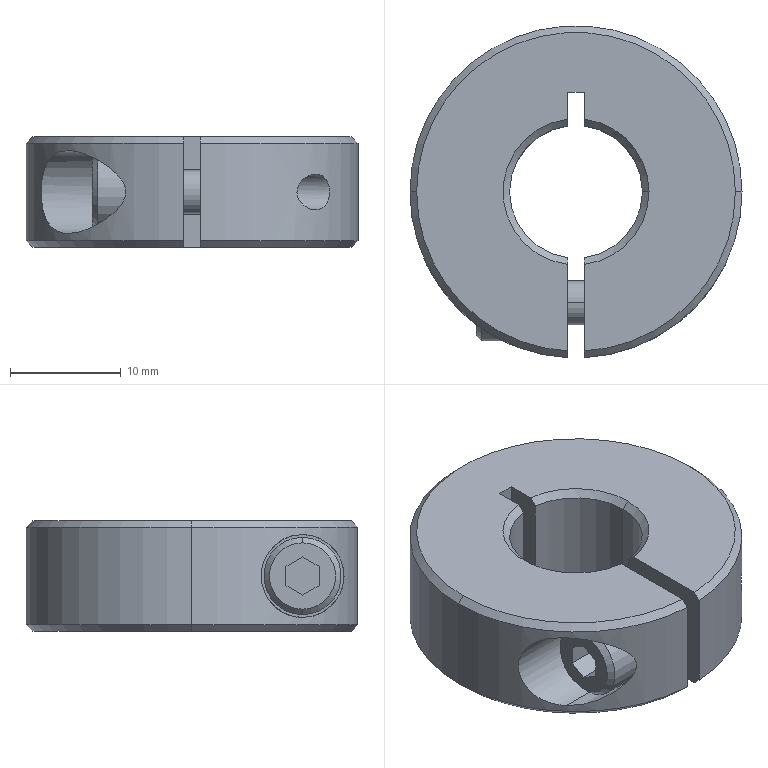Part | NX | features BREP 1 | 1 solid | 50 faces | box 30 x 29.981 x 10 mm | volume 5567 mm3 | plane 18 | cone 16 | cylinder 16 | commonest cylinder face diameters 12 x3 30 x3 3.242 x2 4 x2 4.5 x2 7 x2
STEP:
#1=CARTESIAN_POINT('',(9.,-10.,6.571));
#2=VERTEX_POINT('',#1);
#3=CARTESIAN_POINT('',(9.,-10.,3.429));
#4=VERTEX_POINT('',#3);
#5=CARTESIAN_POINT('',(9.,-10.,5.));
#6=DIRECTION('',(-1.,0.,0.));
#7=DIRECTION('',(0.,0.,1.));
#8=AXIS2_PLACEMENT_3D('',#5,#6,#7);
#9=CIRCLE('',#8,1.571);
#10=EDGE_CURVE('',#2,#4,#9,.T.);
#11=ORIENTED_EDGE('',*,*,#10,.T.);
#12=CARTESIAN_POINT('',(8.95,-10.,3.379));
#13=VERTEX_POINT('',#12);
#14=CARTESIAN_POINT('',(9.,-10.,3.429));
#15=DIRECTION('',(-0.7071,0.,-0.7071));
#16=VECTOR('',#15,1000.);
#17=LINE('',#14,#16);
#18=EDGE_CURVE('',#4,#13,#17,.T.);
#19=ORIENTED_EDGE('',*,*,#18,.T.);
#20=CARTESIAN_POINT('',(8.95,-10.,6.621));
#21=VERTEX_POINT('',#20);
#22=CARTESIAN_POINT('',(8.95,-10.,5.));
#23=DIRECTION('',(-1.,0.,0.));
#24=DIRECTION('',(0.,0.,1.));
#25=AXIS2_PLACEMENT_3D('',#22,#23,#24);
#26=CIRCLE('',#25,1.621);
#27=EDGE_CURVE('',#21,#13,#26,.T.);
#28=ORIENTED_EDGE('',*,*,#27,.F.);
#29=CARTESIAN_POINT('',(9.,-10.,6.571));
#30=DIRECTION('',(-0.7071,0.,0.7071));
#31=VECTOR('',#30,1000.);
#32=LINE('',#29,#31);
#33=EDGE_CURVE('',#2,#21,#32,.T.);
#34=ORIENTED_EDGE('',*,*,#33,.F.);
#35=EDGE_LOOP('',(#11,#19,#28,#34));
#36=FACE_BOUND('',#35,.T.);
#37=CARTESIAN_POINT('',(9.,-10.,5.));
#38=DIRECTION('',(-1.,0.,0.));
#39=DIRECTION('',(0.,0.,-1.));
#40=AXIS2_PLACEMENT_3D('',#37,#38,#39);
#41=CONICAL_SURFACE('',#40,1.571,0.7854);
#42=ADVANCED_FACE('',(#36),#41,.T.);
#43=CARTESIAN_POINT('',(-9.,-10.,8.));
#44=VERTEX_POINT('',#43);
#45=CARTESIAN_POINT('',(-9.,-10.,2.));
#46=VERTEX_POINT('',#45);
#47=CARTESIAN_POINT('',(-9.,-10.,5.));
#48=DIRECTION('',(-1.,0.,0.));
#49=DIRECTION('',(0.,0.,1.));
#50=AXIS2_PLACEMENT_3D('',#47,#48,#49);
#51=CIRCLE('',#50,3.);
#52=EDGE_CURVE('',#44,#46,#51,.T.);
#53=ORIENTED_EDGE('',*,*,#52,.F.);
#54=CARTESIAN_POINT('',(-8.5,-10.,8.5));
#55=VERTEX_POINT('',#54);
#56=CARTESIAN_POINT('',(-8.5,-10.,8.5));
#57=DIRECTION('',(0.7071,0.,0.7071));
#58=VECTOR('',#57,1000.);
#59=LINE('',#56,#58);
#60=EDGE_CURVE('',#55,#44,#59,.F.);
#61=ORIENTED_EDGE('',*,*,#60,.F.);
#62=CARTESIAN_POINT('',(-8.5,-10.,1.5));
#63=VERTEX_POINT('',#62);
#64=CARTESIAN_POINT('',(-8.5,-10.,5.));
#65=DIRECTION('',(-1.,0.,0.));
#66=DIRECTION('',(0.,0.,1.));
#67=AXIS2_PLACEMENT_3D('',#64,#65,#66);
#68=CIRCLE('',#67,3.5);
#69=EDGE_CURVE('',#55,#63,#68,.T.);
#70=ORIENTED_EDGE('',*,*,#69,.T.);
#71=CARTESIAN_POINT('',(-8.5,-10.,1.5));
#72=DIRECTION('',(0.7071,0.,-0.7071));
#73=VECTOR('',#72,1000.);
#74=LINE('',#71,#73);
#75=EDGE_CURVE('',#63,#46,#74,.F.);
#76=ORIENTED_EDGE('',*,*,#75,.T.);
#77=EDGE_LOOP('',(#53,#61,#70,#76));
#78=FACE_BOUND('',#77,.T.);
#79=CARTESIAN_POINT('',(-8.5,-10.,5.));
#80=DIRECTION('',(1.,0.,0.));
#81=DIRECTION('',(0.,0.,1.));
#82=AXIS2_PLACEMENT_3D('',#79,#80,#81);
#83=CONICAL_SURFACE('',#82,3.5,0.7854);
#84=ADVANCED_FACE('',(#78),#83,.T.);
#85=CARTESIAN_POINT('',(-5.,-10.,8.5));
#86=VERTEX_POINT('',#85);
#87=CARTESIAN_POINT('',(-5.,-10.,1.5));
#88=VERTEX_POINT('',#87);
#89=CARTESIAN_POINT('',(-5.,-10.,5.));
#90=DIRECTION('',(-1.,0.,0.));
#91=DIRECTION('',(0.,0.,1.));
#92=AXIS2_PLACEMENT_3D('',#89,#90,#91);
#93=CIRCLE('',#92,3.5);
#94=EDGE_CURVE('',#86,#88,#93,.T.);
#95=ORIENTED_EDGE('',*,*,#94,.T.);
#96=CARTESIAN_POINT('',(50.,-10.,1.5));
#97=DIRECTION('',(-1.,0.,0.));
#98=VECTOR('',#97,1000.);
#99=LINE('',#96,#98);
#100=EDGE_CURVE('',#88,#63,#99,.T.);
#101=ORIENTED_EDGE('',*,*,#100,.T.);
#102=ORIENTED_EDGE('',*,*,#69,.F.);
#103=CARTESIAN_POINT('',(50.,-10.,8.5));
#104=DIRECTION('',(-1.,0.,0.));
#105=VECTOR('',#104,1000.);
#106=LINE('',#103,#105);
#107=EDGE_CURVE('',#86,#55,#106,.T.);
#108=ORIENTED_EDGE('',*,*,#107,.F.);
#109=EDGE_LOOP('',(#95,#101,#102,#108));
#110=FACE_BOUND('',#109,.T.);
#111=CARTESIAN_POINT('',(50.,-10.,5.));
#112=DIRECTION('',(-1.,0.,0.));
#113=DIRECTION('',(0.,0.,-1.));
#114=AXIS2_PLACEMENT_3D('',#111,#112,#113);
#115=CYLINDRICAL_SURFACE('',#114,3.5);
#116=ADVANCED_FACE('',(#110),#115,.T.);
#117=CARTESIAN_POINT('',(0.75,-10.,3.));
#118=VERTEX_POINT('',#117);
#119=CARTESIAN_POINT('',(0.75,-10.,7.));
#120=VERTEX_POINT('',#119);
#121=CARTESIAN_POINT('',(0.75,-10.,5.));
#122=DIRECTION('',(1.,0.,0.));
#123=DIRECTION('',(0.,0.,1.));
#124=AXIS2_PLACEMENT_3D('',#121,#122,#123);
#125=CIRCLE('',#124,2.);
#126=EDGE_CURVE('',#118,#120,#125,.T.);
#127=ORIENTED_EDGE('',*,*,#126,.F.);
#128=CARTESIAN_POINT('',(-5.,-10.,3.));
#129=VERTEX_POINT('',#128);
#130=CARTESIAN_POINT('',(50.,-10.,3.));
#131=DIRECTION('',(-1.,0.,0.));
#132=VECTOR('',#131,1000.);
#133=LINE('',#130,#132);
#134=EDGE_CURVE('',#118,#129,#133,.T.);
#135=ORIENTED_EDGE('',*,*,#134,.T.);
#136=CARTESIAN_POINT('',(-5.,-10.,7.));
#137=VERTEX_POINT('',#136);
#138=CARTESIAN_POINT('',(-5.,-10.,5.));
#139=DIRECTION('',(-1.,0.,0.));
#140=DIRECTION('',(0.,0.,1.));
#141=AXIS2_PLACEMENT_3D('',#138,#139,#140);
#142=CIRCLE('',#141,2.);
#143=EDGE_CURVE('',#137,#129,#142,.T.);
#144=ORIENTED_EDGE('',*,*,#143,.F.);
#145=CARTESIAN_POINT('',(50.,-10.,7.));
#146=DIRECTION('',(-1.,0.,0.));
#147=VECTOR('',#146,1000.);
#148=LINE('',#145,#147);
#149=EDGE_CURVE('',#120,#137,#148,.T.);
#150=ORIENTED_EDGE('',*,*,#149,.F.);
#151=EDGE_LOOP('',(#127,#135,#144,#150));
#152=FACE_BOUND('',#151,.T.);
#153=CARTESIAN_POINT('',(50.,-10.,5.));
#154=DIRECTION('',(-1.,0.,0.));
#155=DIRECTION('',(0.,0.,-1.));
#156=AXIS2_PLACEMENT_3D('',#153,#154,#155);
#157=CYLINDRICAL_SURFACE('',#156,2.);
#158=ADVANCED_FACE('',(#152),#157,.T.);
#159=CARTESIAN_POINT('',(-0.75,-10.,2.75));
#160=VERTEX_POINT('',#159);
#161=CARTESIAN_POINT('',(-0.75,-10.,7.25));
#162=VERTEX_POINT('',#161);
#163=CARTESIAN_POINT('',(-0.75,-10.,5.));
#164=DIRECTION('',(-1.,0.,0.));
#165=DIRECTION('',(0.,0.,-1.));
#166=AXIS2_PLACEMENT_3D('',#163,#164,#165);
#167=CIRCLE('',#166,2.25);
#168=EDGE_CURVE('',#160,#162,#167,.T.);
#169=ORIENTED_EDGE('',*,*,#168,.F.);
#170=CARTESIAN_POINT('',(-5.,-10.,2.75));
#171=VERTEX_POINT('',#170);
#172=CARTESIAN_POINT('',(0.,-10.,2.75));
#173=DIRECTION('',(-1.,0.,0.));
#174=VECTOR('',#173,1000.);
#175=LINE('',#172,#174);
#176=EDGE_CURVE('',#160,#171,#175,.T.);
#177=ORIENTED_EDGE('',*,*,#176,.T.);
#178=CARTESIAN_POINT('',(-5.,-10.,7.25));
#179=VERTEX_POINT('',#178);
#180=CARTESIAN_POINT('',(-5.,-10.,5.));
#181=DIRECTION('',(-1.,0.,0.));
#182=DIRECTION('',(0.,0.,1.));
#183=AXIS2_PLACEMENT_3D('',#180,#181,#182);
#184=CIRCLE('',#183,2.25);
#185=EDGE_CURVE('',#171,#179,#184,.T.);
#186=ORIENTED_EDGE('',*,*,#185,.T.);
#187=CARTESIAN_POINT('',(0.,-10.,7.25));
#188=DIRECTION('',(-1.,0.,0.));
#189=VECTOR('',#188,1000.);
#190=LINE('',#187,#189);
#191=EDGE_CURVE('',#162,#179,#190,.T.);
#192=ORIENTED_EDGE('',*,*,#191,.F.);
#193=EDGE_LOOP('',(#169,#177,#186,#192));
#194=FACE_BOUND('',#193,.T.);
#195=CARTESIAN_POINT('',(0.,-10.,5.));
#196=DIRECTION('',(-1.,0.,0.));
#197=DIRECTION('',(0.,0.,-1.));
#198=AXIS2_PLACEMENT_3D('',#195,#196,#197);
#199=CYLINDRICAL_SURFACE('',#198,2.25);
#200=ADVANCED_FACE('',(#194),#199,.F.);
#201=CARTESIAN_POINT('',(-5.,-10.,1.25));
#202=VERTEX_POINT('',#201);
#203=CARTESIAN_POINT('',(-5.,-10.,8.75));
#204=VERTEX_POINT('',#203);
#205=CARTESIAN_POINT('',(-5.,-10.,5.));
#206=DIRECTION('',(-1.,0.,0.));
#207=DIRECTION('',(0.,0.,1.));
#208=AXIS2_PLACEMENT_3D('',#205,#206,#207);
#209=CIRCLE('',#208,3.75);
#210=EDGE_CURVE('',#202,#204,#209,.T.);
#211=ORIENTED_EDGE('',*,*,#210,.F.);
#212=CARTESIAN_POINT('',(-11.18,-10.,1.25));
#213=VERTEX_POINT('',#212);
#214=CARTESIAN_POINT('',(0.,-10.,1.25));
#215=DIRECTION('',(-1.,0.,0.));
#216=VECTOR('',#215,1000.);
#217=LINE('',#214,#216);
#218=EDGE_CURVE('',#202,#213,#217,.T.);
#219=ORIENTED_EDGE('',*,*,#218,.T.);
#220=CARTESIAN_POINT('',(-11.18,-10.,8.75));
#221=VERTEX_POINT('',#220);
#222=CARTESIAN_POINT('',(-11.18,-10.,1.25));
#223=CARTESIAN_POINT('',(-10.734,-10.499,1.25));
#224=CARTESIAN_POINT('',(-9.793,-11.416,1.443));
#225=CARTESIAN_POINT('',(-8.292,-12.544,2.142));
#226=CARTESIAN_POINT('',(-7.049,-13.257,3.035));
#227=CARTESIAN_POINT('',(-6.225,-13.651,4.));
#228=CARTESIAN_POINT('',(-5.882,-13.798,4.991));
#229=CARTESIAN_POINT('',(-6.214,-13.656,5.984));
#230=CARTESIAN_POINT('',(-7.046,-13.259,6.965));
#231=CARTESIAN_POINT('',(-8.287,-12.547,7.853));
#232=CARTESIAN_POINT('',(-9.776,-11.432,8.552));
#233=CARTESIAN_POINT('',(-10.733,-10.5,8.75));
#234=CARTESIAN_POINT('',(-11.18,-10.,8.75));
#235=B_SPLINE_CURVE_WITH_KNOTS('',3,(#222,#223,#224,#225,#226,#227,#228,#229,#230,#231,#232,#233,#234),.UNSPECIFIED.,.F.,.F.,(4,1,1,1,1,1,1,1,1,1,4),(0.,0.001981,0.003961,0.005942,0.006932,0.007922,0.008912,0.009903,0.01188,0.01386,0.01584),.UNSPECIFIED.);
#236=EDGE_CURVE('',#213,#221,#235,.T.);
#237=ORIENTED_EDGE('',*,*,#236,.T.);
#238=CARTESIAN_POINT('',(0.,-10.,8.75));
#239=DIRECTION('',(-1.,0.,0.));
#240=VECTOR('',#239,1000.);
#241=LINE('',#238,#240);
#242=EDGE_CURVE('',#204,#221,#241,.T.);
#243=ORIENTED_EDGE('',*,*,#242,.F.);
#244=EDGE_LOOP('',(#211,#219,#237,#243));
#245=FACE_BOUND('',#244,.T.);
#246=CARTESIAN_POINT('',(0.,-10.,5.));
#247=DIRECTION('',(-1.,0.,0.));
#248=DIRECTION('',(0.,0.,-1.));
#249=AXIS2_PLACEMENT_3D('',#246,#247,#248);
#250=CYLINDRICAL_SURFACE('',#249,3.75);
#251=ADVANCED_FACE('',(#245),#250,.F.);
#252=CARTESIAN_POINT('',(14.4,0.,0.));
#253=VERTEX_POINT('',#252);
#254=CARTESIAN_POINT('',(-14.4,0.,0.));
#255=VERTEX_POINT('',#254);
#256=CARTESIAN_POINT('',(0.,0.,0.));
#257=DIRECTION('',(0.,0.,1.));
#258=DIRECTION('',(1.,0.,0.));
#259=AXIS2_PLACEMENT_3D('',#256,#257,#258);
#260=CIRCLE('',#259,14.4);
#261=EDGE_CURVE('',#253,#255,#260,.T.);
#262=ORIENTED_EDGE('',*,*,#261,.T.);
#263=CARTESIAN_POINT('',(-15.,0.,0.6));
#264=VERTEX_POINT('',#263);
#265=CARTESIAN_POINT('',(-14.4,0.,0.));
#266=DIRECTION('',(-0.7071,0.,0.7071));
#267=VECTOR('',#266,1000.);
#268=LINE('',#265,#267);
#269=EDGE_CURVE('',#255,#264,#268,.T.);
#270=ORIENTED_EDGE('',*,*,#269,.T.);
#271=CARTESIAN_POINT('',(15.,0.,0.6));
#272=VERTEX_POINT('',#271);
#273=CARTESIAN_POINT('',(0.,0.,0.6));
#274=DIRECTION('',(0.,0.,1.));
#275=DIRECTION('',(1.,0.,0.));
#276=AXIS2_PLACEMENT_3D('',#273,#274,#275);
#277=CIRCLE('',#276,15.);
#278=EDGE_CURVE('',#272,#264,#277,.T.);
#279=ORIENTED_EDGE('',*,*,#278,.F.);
#280=CARTESIAN_POINT('',(14.4,0.,0.));
#281=DIRECTION('',(0.7071,0.,0.7071));
#282=VECTOR('',#281,1000.);
#283=LINE('',#280,#282);
#284=EDGE_CURVE('',#253,#272,#283,.T.);
#285=ORIENTED_EDGE('',*,*,#284,.F.);
#286=EDGE_LOOP('',(#262,#270,#279,#285));
#287=FACE_BOUND('',#286,.T.);
#288=CARTESIAN_POINT('',(0.,0.,0.));
#289=DIRECTION('',(0.,0.,1.));
#290=DIRECTION('',(-1.,0.,0.));
#291=AXIS2_PLACEMENT_3D('',#288,#289,#290);
#292=CONICAL_SURFACE('',#291,14.4,0.7854);
#293=ADVANCED_FACE('',(#287),#292,.T.);
#294=CARTESIAN_POINT('',(0.75,-14.38,0.));
#295=VERTEX_POINT('',#294);
#296=CARTESIAN_POINT('',(0.,0.,0.));
#297=DIRECTION('',(0.,0.,1.));
#298=DIRECTION('',(1.,0.,0.));
#299=AXIS2_PLACEMENT_3D('',#296,#297,#298);
#300=CIRCLE('',#299,14.4);
#301=EDGE_CURVE('',#295,#253,#300,.T.);
#302=ORIENTED_EDGE('',*,*,#301,.T.);
#303=ORIENTED_EDGE('',*,*,#284,.T.);
#304=CARTESIAN_POINT('',(0.75,-14.981,0.6));
#305=VERTEX_POINT('',#304);
#306=CARTESIAN_POINT('',(0.,0.,0.6));
#307=DIRECTION('',(0.,0.,1.));
#308=DIRECTION('',(1.,0.,0.));
#309=AXIS2_PLACEMENT_3D('',#306,#307,#308);
#310=CIRCLE('',#309,15.);
#311=EDGE_CURVE('',#305,#272,#310,.T.);
#312=ORIENTED_EDGE('',*,*,#311,.F.);
#313=CARTESIAN_POINT('',(0.75,-14.38,0.));
#314=CARTESIAN_POINT('',(0.75,-14.581,0.2));
#315=CARTESIAN_POINT('',(0.75,-14.781,0.4));
#316=CARTESIAN_POINT('',(0.75,-14.981,0.6));
#317=B_SPLINE_CURVE_WITH_KNOTS('',3,(#313,#314,#315,#316),.UNSPECIFIED.,.F.,.F.,(4,4),(0.,1.),.PIECEWISE_BEZIER_KNOTS.);
#318=EDGE_CURVE('',#295,#305,#317,.T.);
#319=ORIENTED_EDGE('',*,*,#318,.F.);
#320=EDGE_LOOP('',(#302,#303,#312,#319));
#321=FACE_BOUND('',#320,.T.);
#322=CARTESIAN_POINT('',(0.,0.,0.));
#323=DIRECTION('',(0.,0.,1.));
#324=DIRECTION('',(-1.,0.,0.));
#325=AXIS2_PLACEMENT_3D('',#322,#323,#324);
#326=CONICAL_SURFACE('',#325,14.4,0.7854);
#327=ADVANCED_FACE('',(#321),#326,.T.);
#328=CARTESIAN_POINT('',(-0.75,5.953,0.6));
#329=VERTEX_POINT('',#328);
#330=CARTESIAN_POINT('',(-6.,0.,0.6));
#331=VERTEX_POINT('',#330);
#332=CARTESIAN_POINT('',(0.,0.,0.6));
#333=DIRECTION('',(0.,0.,1.));
#334=DIRECTION('',(1.,0.,0.));
#335=AXIS2_PLACEMENT_3D('',#332,#333,#334);
#336=CIRCLE('',#335,6.);
#337=EDGE_CURVE('',#329,#331,#336,.T.);
#338=ORIENTED_EDGE('',*,*,#337,.T.);
#339=CARTESIAN_POINT('',(-6.6,0.,0.));
#340=VERTEX_POINT('',#339);
#341=CARTESIAN_POINT('',(-6.,0.,0.6));
#342=DIRECTION('',(-0.7071,0.,-0.7071));
#343=VECTOR('',#342,1000.);
#344=LINE('',#341,#343);
#345=EDGE_CURVE('',#331,#340,#344,.T.);
#346=ORIENTED_EDGE('',*,*,#345,.T.);
#347=CARTESIAN_POINT('',(-0.75,6.557,0.));
#348=VERTEX_POINT('',#347);
#349=CARTESIAN_POINT('',(0.,0.,0.));
#350=DIRECTION('',(0.,0.,1.));
#351=DIRECTION('',(1.,0.,0.));
#352=AXIS2_PLACEMENT_3D('',#349,#350,#351);
#353=CIRCLE('',#352,6.6);
#354=EDGE_CURVE('',#348,#340,#353,.T.);
#355=ORIENTED_EDGE('',*,*,#354,.F.);
#356=CARTESIAN_POINT('',(-0.75,5.953,0.6));
#357=CARTESIAN_POINT('',(-0.75,6.154,0.4001));
#358=CARTESIAN_POINT('',(-0.75,6.356,0.2001));
#359=CARTESIAN_POINT('',(-0.75,6.557,0.));
#360=B_SPLINE_CURVE_WITH_KNOTS('',3,(#356,#357,#358,#359),.UNSPECIFIED.,.F.,.F.,(4,4),(0.,1.),.PIECEWISE_BEZIER_KNOTS.);
#361=EDGE_CURVE('',#329,#348,#360,.T.);
#362=ORIENTED_EDGE('',*,*,#361,.F.);
#363=EDGE_LOOP('',(#338,#346,#355,#362));
#364=FACE_BOUND('',#363,.T.);
#365=CARTESIAN_POINT('',(0.,0.,0.6));
#366=DIRECTION('',(0.,0.,-1.));
#367=DIRECTION('',(1.,0.,0.));
#368=AXIS2_PLACEMENT_3D('',#365,#366,#367);
#369=CONICAL_SURFACE('',#368,6.,0.7854);
#370=ADVANCED_FACE('',(#364),#369,.F.);
#371=CARTESIAN_POINT('',(6.,0.,0.6));
#372=VERTEX_POINT('',#371);
#373=CARTESIAN_POINT('',(0.75,5.953,0.6));
#374=VERTEX_POINT('',#373);
#375=CARTESIAN_POINT('',(0.,0.,0.6));
#376=DIRECTION('',(0.,0.,1.));
#377=DIRECTION('',(1.,0.,0.));
#378=AXIS2_PLACEMENT_3D('',#375,#376,#377);
#379=CIRCLE('',#378,6.);
#380=EDGE_CURVE('',#372,#374,#379,.T.);
#381=ORIENTED_EDGE('',*,*,#380,.F.);
#382=CARTESIAN_POINT('',(6.,0.,9.4));
#383=VERTEX_POINT('',#382);
#384=CARTESIAN_POINT('',(6.,0.,0.));
#385=DIRECTION('',(0.,0.,1.));
#386=VECTOR('',#385,1000.);
#387=LINE('',#384,#386);
#388=EDGE_CURVE('',#372,#383,#387,.T.);
#389=ORIENTED_EDGE('',*,*,#388,.T.);
#390=CARTESIAN_POINT('',(0.75,5.953,9.4));
#391=VERTEX_POINT('',#390);
#392=CARTESIAN_POINT('',(0.,0.,9.4));
#393=DIRECTION('',(0.,0.,1.));
#394=DIRECTION('',(1.,0.,0.));
#395=AXIS2_PLACEMENT_3D('',#392,#393,#394);
#396=CIRCLE('',#395,6.);
#397=EDGE_CURVE('',#383,#391,#396,.T.);
#398=ORIENTED_EDGE('',*,*,#397,.T.);
#399=CARTESIAN_POINT('',(0.75,5.953,0.));
#400=DIRECTION('',(0.,0.,1.));
#401=VECTOR('',#400,1000.);
#402=LINE('',#399,#401);
#403=EDGE_CURVE('',#374,#391,#402,.T.);
#404=ORIENTED_EDGE('',*,*,#403,.F.);
#405=EDGE_LOOP('',(#381,#389,#398,#404));
#406=FACE_BOUND('',#405,.T.);
#407=CARTESIAN_POINT('',(0.,0.,0.));
#408=DIRECTION('',(0.,0.,1.));
#409=DIRECTION('',(-1.,0.,0.));
#410=AXIS2_PLACEMENT_3D('',#407,#408,#409);
#411=CYLINDRICAL_SURFACE('',#410,6.);
#412=ADVANCED_FACE('',(#406),#411,.F.);
#413=ORIENTED_EDGE('',*,*,#397,.F.);
#414=CARTESIAN_POINT('',(6.6,0.,10.));
#415=VERTEX_POINT('',#414);
#416=CARTESIAN_POINT('',(6.6,0.,10.));
#417=DIRECTION('',(0.7071,0.,0.7071));
#418=VECTOR('',#417,1000.);
#419=LINE('',#416,#418);
#420=EDGE_CURVE('',#383,#415,#419,.T.);
#421=ORIENTED_EDGE('',*,*,#420,.T.);
#422=CARTESIAN_POINT('',(0.75,6.557,10.));
#423=VERTEX_POINT('',#422);
#424=CARTESIAN_POINT('',(0.,0.,10.));
#425=DIRECTION('',(0.,0.,1.));
#426=DIRECTION('',(1.,0.,0.));
#427=AXIS2_PLACEMENT_3D('',#424,#425,#426);
#428=CIRCLE('',#427,6.6);
#429=EDGE_CURVE('',#415,#423,#428,.T.);
#430=ORIENTED_EDGE('',*,*,#429,.T.);
#431=CARTESIAN_POINT('',(0.75,5.953,9.4));
#432=CARTESIAN_POINT('',(0.75,6.154,9.6));
#433=CARTESIAN_POINT('',(0.75,6.356,9.8));
#434=CARTESIAN_POINT('',(0.75,6.557,10.));
#435=B_SPLINE_CURVE_WITH_KNOTS('',3,(#431,#432,#433,#434),.UNSPECIFIED.,.F.,.F.,(4,4),(0.,1.),.PIECEWISE_BEZIER_KNOTS.);
#436=EDGE_CURVE('',#391,#423,#435,.T.);
#437=ORIENTED_EDGE('',*,*,#436,.F.);
#438=EDGE_LOOP('',(#413,#421,#430,#437));
#439=FACE_BOUND('',#438,.T.);
#440=CARTESIAN_POINT('',(0.,0.,10.));
#441=DIRECTION('',(0.,0.,1.));
#442=DIRECTION('',(-1.,0.,0.));
#443=AXIS2_PLACEMENT_3D('',#440,#441,#442);
#444=CONICAL_SURFACE('',#443,6.6,0.7854);
#445=ADVANCED_FACE('',(#439),#444,.F.);
#446=CARTESIAN_POINT('',(14.4,0.,10.));
#447=VERTEX_POINT('',#446);
#448=CARTESIAN_POINT('',(-14.4,0.,10.));
#449=VERTEX_POINT('',#448);
#450=CARTESIAN_POINT('',(0.,0.,10.));
#451=DIRECTION('',(0.,0.,1.));
#452=DIRECTION('',(1.,0.,0.));
#453=AXIS2_PLACEMENT_3D('',#450,#451,#452);
#454=CIRCLE('',#453,14.4);
#455=EDGE_CURVE('',#447,#449,#454,.T.);
#456=ORIENTED_EDGE('',*,*,#455,.F.);
#457=CARTESIAN_POINT('',(15.,0.,9.4));
#458=VERTEX_POINT('',#457);
#459=CARTESIAN_POINT('',(15.,0.,9.4));
#460=DIRECTION('',(0.7071,0.,-0.7071));
#461=VECTOR('',#460,1000.);
#462=LINE('',#459,#461);
#463=EDGE_CURVE('',#447,#458,#462,.T.);
#464=ORIENTED_EDGE('',*,*,#463,.T.);
#465=CARTESIAN_POINT('',(-15.,0.,9.4));
#466=VERTEX_POINT('',#465);
#467=CARTESIAN_POINT('',(0.,0.,9.4));
#468=DIRECTION('',(0.,0.,1.));
#469=DIRECTION('',(1.,0.,0.));
#470=AXIS2_PLACEMENT_3D('',#467,#468,#469);
#471=CIRCLE('',#470,15.);
#472=EDGE_CURVE('',#458,#466,#471,.T.);
#473=ORIENTED_EDGE('',*,*,#472,.T.);
#474=CARTESIAN_POINT('',(-15.,0.,9.4));
#475=DIRECTION('',(-0.7071,0.,-0.7071));
#476=VECTOR('',#475,1000.);
#477=LINE('',#474,#476);
#478=EDGE_CURVE('',#449,#466,#477,.T.);
#479=ORIENTED_EDGE('',*,*,#478,.F.);
#480=EDGE_LOOP('',(#456,#464,#473,#479));
#481=FACE_BOUND('',#480,.T.);
#482=CARTESIAN_POINT('',(0.,0.,9.4));
#483=DIRECTION('',(0.,0.,-1.));
#484=DIRECTION('',(1.,0.,0.));
#485=AXIS2_PLACEMENT_3D('',#482,#483,#484);
#486=CONICAL_SURFACE('',#485,15.,0.7854);
#487=ADVANCED_FACE('',(#481),#486,.T.);
#488=CARTESIAN_POINT('',(-0.75,-14.38,10.));
#489=VERTEX_POINT('',#488);
#490=CARTESIAN_POINT('',(0.,0.,10.));
#491=DIRECTION('',(0.,0.,1.));
#492=DIRECTION('',(1.,0.,0.));
#493=AXIS2_PLACEMENT_3D('',#490,#491,#492);
#494=CIRCLE('',#493,14.4);
#495=EDGE_CURVE('',#449,#489,#494,.T.);
#496=ORIENTED_EDGE('',*,*,#495,.F.);
#497=ORIENTED_EDGE('',*,*,#478,.T.);
#498=CARTESIAN_POINT('',(-0.75,-14.981,9.4));
#499=VERTEX_POINT('',#498);
#500=CARTESIAN_POINT('',(0.,0.,9.4));
#501=DIRECTION('',(0.,0.,1.));
#502=DIRECTION('',(1.,0.,0.));
#503=AXIS2_PLACEMENT_3D('',#500,#501,#502);
#504=CIRCLE('',#503,15.);
#505=EDGE_CURVE('',#466,#499,#504,.T.);
#506=ORIENTED_EDGE('',*,*,#505,.T.);
#507=CARTESIAN_POINT('',(-0.75,-14.38,10.));
#508=CARTESIAN_POINT('',(-0.75,-14.581,9.8));
#509=CARTESIAN_POINT('',(-0.75,-14.781,9.6));
#510=CARTESIAN_POINT('',(-0.75,-14.981,9.4));
#511=B_SPLINE_CURVE_WITH_KNOTS('',3,(#507,#508,#509,#510),.UNSPECIFIED.,.F.,.F.,(4,4),(0.,1.),.PIECEWISE_BEZIER_KNOTS.);
#512=EDGE_CURVE('',#489,#499,#511,.T.);
#513=ORIENTED_EDGE('',*,*,#512,.F.);
#514=EDGE_LOOP('',(#496,#497,#506,#513));
#515=FACE_BOUND('',#514,.T.);
#516=CARTESIAN_POINT('',(0.,0.,9.4));
#517=DIRECTION('',(0.,0.,-1.));
#518=DIRECTION('',(1.,0.,0.));
#519=AXIS2_PLACEMENT_3D('',#516,#517,#518);
#520=CONICAL_SURFACE('',#519,15.,0.7854);
#521=ADVANCED_FACE('',(#515),#520,.T.);
#522=ORIENTED_EDGE('',*,*,#278,.T.);
#523=CARTESIAN_POINT('',(-15.,0.,0.));
#524=DIRECTION('',(0.,0.,1.));
#525=VECTOR('',#524,1000.);
#526=LINE('',#523,#525);
#527=EDGE_CURVE('',#264,#466,#526,.T.);
#528=ORIENTED_EDGE('',*,*,#527,.T.);
#529=ORIENTED_EDGE('',*,*,#472,.F.);
#530=CARTESIAN_POINT('',(15.,0.,0.));
#531=DIRECTION('',(0.,0.,1.));
#532=VECTOR('',#531,1000.);
#533=LINE('',#530,#532);
#534=EDGE_CURVE('',#272,#458,#533,.T.);
#535=ORIENTED_EDGE('',*,*,#534,.F.);
#536=EDGE_LOOP('',(#522,#528,#529,#535));
#537=FACE_BOUND('',#536,.T.);
#538=CARTESIAN_POINT('',(0.,0.,0.));
#539=DIRECTION('',(0.,0.,1.));
#540=DIRECTION('',(-1.,0.,0.));
#541=AXIS2_PLACEMENT_3D('',#538,#539,#540);
#542=CYLINDRICAL_SURFACE('',#541,15.);
#543=ADVANCED_FACE('',(#537),#542,.T.);
#544=CARTESIAN_POINT('',(11.18,-10.,3.379));
#545=VERTEX_POINT('',#544);
#546=CARTESIAN_POINT('',(11.18,-10.,6.621));
#547=VERTEX_POINT('',#546);
#548=CARTESIAN_POINT('',(11.18,-10.,3.379));
#549=CARTESIAN_POINT('',(11.505,-9.637,3.379));
#550=CARTESIAN_POINT('',(12.121,-8.866,3.599));
#551=CARTESIAN_POINT('',(12.601,-8.137,4.992));
#552=CARTESIAN_POINT('',(12.126,-8.858,6.399));
#553=CARTESIAN_POINT('',(11.506,-9.636,6.621));
#554=CARTESIAN_POINT('',(11.18,-10.,6.621));
#555=B_SPLINE_CURVE_WITH_KNOTS('',3,(#548,#549,#550,#551,#552,#553,#554),.UNSPECIFIED.,.F.,.F.,(4,1,1,1,4),(0.,0.001443,0.002887,0.00433,0.005774),.UNSPECIFIED.);
#556=EDGE_CURVE('',#545,#547,#555,.T.);
#557=ORIENTED_EDGE('',*,*,#556,.F.);
#558=CARTESIAN_POINT('',(11.18,-10.,6.621));
#559=CARTESIAN_POINT('',(10.831,-10.391,6.621));
#560=CARTESIAN_POINT('',(10.284,-10.937,6.423));
#561=CARTESIAN_POINT('',(9.653,-11.485,5.77));
#562=CARTESIAN_POINT('',(9.401,-11.689,5.003));
#563=CARTESIAN_POINT('',(9.651,-11.486,4.232));
#564=CARTESIAN_POINT('',(10.28,-10.94,3.579));
#565=CARTESIAN_POINT('',(10.831,-10.39,3.379));
#566=CARTESIAN_POINT('',(11.18,-10.,3.379));
#567=B_SPLINE_CURVE_WITH_KNOTS('',3,(#558,#559,#560,#561,#562,#563,#564,#565,#566),.UNSPECIFIED.,.F.,.F.,(4,1,1,1,1,1,4),(0.,0.00155,0.002325,0.0031,0.003875,0.00465,0.0062),.UNSPECIFIED.);
#568=EDGE_CURVE('',#547,#545,#567,.T.);
#569=ORIENTED_EDGE('',*,*,#568,.F.);
#570=EDGE_LOOP('',(#557,#569));
#571=FACE_BOUND('',#570,.T.);
#572=ORIENTED_EDGE('',*,*,#311,.T.);
#573=ORIENTED_EDGE('',*,*,#534,.T.);
#574=CARTESIAN_POINT('',(0.75,-14.981,9.4));
#575=VERTEX_POINT('',#574);
#576=CARTESIAN_POINT('',(0.,0.,9.4));
#577=DIRECTION('',(0.,0.,1.));
#578=DIRECTION('',(1.,0.,0.));
#579=AXIS2_PLACEMENT_3D('',#576,#577,#578);
#580=CIRCLE('',#579,15.);
#581=EDGE_CURVE('',#575,#458,#580,.T.);
#582=ORIENTED_EDGE('',*,*,#581,.F.);
#583=CARTESIAN_POINT('',(0.75,-14.981,0.));
#584=DIRECTION('',(0.,0.,1.));
#585=VECTOR('',#584,1000.);
#586=LINE('',#583,#585);
#587=EDGE_CURVE('',#305,#575,#586,.T.);
#588=ORIENTED_EDGE('',*,*,#587,.F.);
#589=EDGE_LOOP('',(#572,#573,#582,#588));
#590=FACE_BOUND('',#589,.T.);
#591=CARTESIAN_POINT('',(0.,0.,0.));
#592=DIRECTION('',(0.,0.,1.));
#593=DIRECTION('',(-1.,0.,0.));
#594=AXIS2_PLACEMENT_3D('',#591,#592,#593);
#595=CYLINDRICAL_SURFACE('',#594,15.);
#596=ADVANCED_FACE('',(#571,#590),#595,.T.);
#597=CARTESIAN_POINT('',(8.95,-10.,5.));
#598=DIRECTION('',(-1.,0.,0.));
#599=DIRECTION('',(0.,0.,1.));
#600=AXIS2_PLACEMENT_3D('',#597,#598,#599);
#601=CIRCLE('',#600,1.621);
#602=EDGE_CURVE('',#13,#21,#601,.T.);
#603=ORIENTED_EDGE('',*,*,#602,.T.);
#604=CARTESIAN_POINT('',(0.,-10.,6.621));
#605=DIRECTION('',(1.,0.,0.));
#606=VECTOR('',#605,1000.);
#607=LINE('',#604,#606);
#608=EDGE_CURVE('',#547,#21,#607,.F.);
#609=ORIENTED_EDGE('',*,*,#608,.F.);
#610=ORIENTED_EDGE('',*,*,#568,.T.);
#611=CARTESIAN_POINT('',(0.,-10.,3.379));
#612=DIRECTION('',(1.,0.,0.));
#613=VECTOR('',#612,1000.);
#614=LINE('',#611,#613);
#615=EDGE_CURVE('',#545,#13,#614,.F.);
#616=ORIENTED_EDGE('',*,*,#615,.T.);
#617=EDGE_LOOP('',(#603,#609,#610,#616));
#618=FACE_BOUND('',#617,.T.);
#619=CARTESIAN_POINT('',(0.,-10.,5.));
#620=DIRECTION('',(1.,0.,0.));
#621=DIRECTION('',(0.,0.,1.));
#622=AXIS2_PLACEMENT_3D('',#619,#620,#621);
#623=CYLINDRICAL_SURFACE('',#622,1.621);
#624=ADVANCED_FACE('',(#618),#623,.F.);
#625=ORIENTED_EDGE('',*,*,#608,.T.);
#626=ORIENTED_EDGE('',*,*,#27,.T.);
#627=ORIENTED_EDGE('',*,*,#615,.F.);
#628=ORIENTED_EDGE('',*,*,#556,.T.);
#629=EDGE_LOOP('',(#625,#626,#627,#628));
#630=FACE_BOUND('',#629,.T.);
#631=CARTESIAN_POINT('',(0.,-10.,5.));
#632=DIRECTION('',(1.,0.,0.));
#633=DIRECTION('',(0.,0.,1.));
#634=AXIS2_PLACEMENT_3D('',#631,#632,#633);
#635=CYLINDRICAL_SURFACE('',#634,1.621);
#636=ADVANCED_FACE('',(#630),#635,.F.);
#637=ORIENTED_EDGE('',*,*,#527,.F.);
#638=CARTESIAN_POINT('',(-0.75,-14.981,0.6));
#639=VERTEX_POINT('',#638);
#640=CARTESIAN_POINT('',(0.,0.,0.6));
#641=DIRECTION('',(0.,0.,1.));
#642=DIRECTION('',(1.,0.,0.));
#643=AXIS2_PLACEMENT_3D('',#640,#641,#642);
#644=CIRCLE('',#643,15.);
#645=EDGE_CURVE('',#264,#639,#644,.T.);
#646=ORIENTED_EDGE('',*,*,#645,.T.);
#647=CARTESIAN_POINT('',(-0.75,-14.981,0.));
#648=DIRECTION('',(0.,0.,-1.));
#649=VECTOR('',#648,1000.);
#650=LINE('',#647,#649);
#651=EDGE_CURVE('',#499,#639,#650,.T.);
#652=ORIENTED_EDGE('',*,*,#651,.F.);
#653=ORIENTED_EDGE('',*,*,#505,.F.);
#654=EDGE_LOOP('',(#637,#646,#652,#653));
#655=FACE_BOUND('',#654,.T.);
#656=CARTESIAN_POINT('',(-11.18,-10.,8.75));
#657=CARTESIAN_POINT('',(-11.91,-9.184,8.75));
#658=CARTESIAN_POINT('',(-13.179,-7.332,8.218));
#659=CARTESIAN_POINT('',(-13.861,-5.714,5.017));
#660=CARTESIAN_POINT('',(-13.19,-7.313,1.79));
#661=CARTESIAN_POINT('',(-11.912,-9.182,1.25));
#662=CARTESIAN_POINT('',(-11.18,-10.,1.25));
#663=B_SPLINE_CURVE_WITH_KNOTS('',3,(#656,#657,#658,#659,#660,#661,#662),.UNSPECIFIED.,.F.,.F.,(4,1,1,1,4),(0.,0.003235,0.006471,0.009706,0.01294),.UNSPECIFIED.);
#664=EDGE_CURVE('',#221,#213,#663,.T.);
#665=ORIENTED_EDGE('',*,*,#664,.F.);
#666=ORIENTED_EDGE('',*,*,#236,.F.);
#667=EDGE_LOOP('',(#665,#666));
#668=FACE_BOUND('',#667,.T.);
#669=CARTESIAN_POINT('',(0.,0.,0.));
#670=DIRECTION('',(0.,0.,1.));
#671=DIRECTION('',(-1.,0.,0.));
#672=AXIS2_PLACEMENT_3D('',#669,#670,#671);
#673=CYLINDRICAL_SURFACE('',#672,15.);
#674=ADVANCED_FACE('',(#655,#668),#673,.T.);
#675=ORIENTED_EDGE('',*,*,#463,.F.);
#676=CARTESIAN_POINT('',(0.75,-14.38,10.));
#677=VERTEX_POINT('',#676);
#678=CARTESIAN_POINT('',(0.,0.,10.));
#679=DIRECTION('',(0.,0.,1.));
#680=DIRECTION('',(1.,0.,0.));
#681=AXIS2_PLACEMENT_3D('',#678,#679,#680);
#682=CIRCLE('',#681,14.4);
#683=EDGE_CURVE('',#677,#447,#682,.T.);
#684=ORIENTED_EDGE('',*,*,#683,.F.);
#685=CARTESIAN_POINT('',(0.75,-14.981,9.4));
#686=CARTESIAN_POINT('',(0.75,-14.781,9.6));
#687=CARTESIAN_POINT('',(0.75,-14.581,9.8));
#688=CARTESIAN_POINT('',(0.75,-14.38,10.));
#689=B_SPLINE_CURVE_WITH_KNOTS('',3,(#685,#686,#687,#688),.UNSPECIFIED.,.F.,.F.,(4,4),(0.,1.),.PIECEWISE_BEZIER_KNOTS.);
#690=EDGE_CURVE('',#575,#677,#689,.T.);
#691=ORIENTED_EDGE('',*,*,#690,.F.);
#692=ORIENTED_EDGE('',*,*,#581,.T.);
#693=EDGE_LOOP('',(#675,#684,#691,#692));
#694=FACE_BOUND('',#693,.T.);
#695=CARTESIAN_POINT('',(0.,0.,9.4));
#696=DIRECTION('',(0.,0.,-1.));
#697=DIRECTION('',(1.,0.,0.));
#698=AXIS2_PLACEMENT_3D('',#695,#696,#697);
#699=CONICAL_SURFACE('',#698,15.,0.7854);
#700=ADVANCED_FACE('',(#694),#699,.T.);
#701=CARTESIAN_POINT('',(-0.75,-6.557,10.));
#702=VERTEX_POINT('',#701);
#703=CARTESIAN_POINT('',(-0.75,9.,10.));
#704=DIRECTION('',(0.,-1.,0.));
#705=VECTOR('',#704,1000.);
#706=LINE('',#703,#705);
#707=EDGE_CURVE('',#702,#489,#706,.T.);
#708=ORIENTED_EDGE('',*,*,#707,.F.);
#709=CARTESIAN_POINT('',(-0.75,6.557,10.));
#710=VERTEX_POINT('',#709);
#711=CARTESIAN_POINT('',(0.,0.,10.));
#712=DIRECTION('',(0.,0.,1.));
#713=DIRECTION('',(1.,0.,0.));
#714=AXIS2_PLACEMENT_3D('',#711,#712,#713);
#715=CIRCLE('',#714,6.6);
#716=EDGE_CURVE('',#710,#702,#715,.T.);
#717=ORIENTED_EDGE('',*,*,#716,.F.);
#718=CARTESIAN_POINT('',(-0.75,9.,10.));
#719=VERTEX_POINT('',#718);
#720=CARTESIAN_POINT('',(-0.75,9.,10.));
#721=DIRECTION('',(0.,-1.,0.));
#722=VECTOR('',#721,1000.);
#723=LINE('',#720,#722);
#724=EDGE_CURVE('',#719,#710,#723,.T.);
#725=ORIENTED_EDGE('',*,*,#724,.F.);
#726=CARTESIAN_POINT('',(0.75,9.,10.));
#727=VERTEX_POINT('',#726);
#728=CARTESIAN_POINT('',(0.75,9.,10.));
#729=DIRECTION('',(-1.,0.,0.));
#730=VECTOR('',#729,1000.);
#731=LINE('',#728,#730);
#732=EDGE_CURVE('',#727,#719,#731,.T.);
#733=ORIENTED_EDGE('',*,*,#732,.F.);
#734=CARTESIAN_POINT('',(0.75,-16.,10.));
#735=DIRECTION('',(0.,1.,0.));
#736=VECTOR('',#735,1000.);
#737=LINE('',#734,#736);
#738=EDGE_CURVE('',#423,#727,#737,.T.);
#739=ORIENTED_EDGE('',*,*,#738,.F.);
#740=ORIENTED_EDGE('',*,*,#429,.F.);
#741=CARTESIAN_POINT('',(0.75,-6.557,10.));
#742=VERTEX_POINT('',#741);
#743=CARTESIAN_POINT('',(0.,0.,10.));
#744=DIRECTION('',(0.,0.,1.));
#745=DIRECTION('',(1.,0.,0.));
#746=AXIS2_PLACEMENT_3D('',#743,#744,#745);
#747=CIRCLE('',#746,6.6);
#748=EDGE_CURVE('',#742,#415,#747,.T.);
#749=ORIENTED_EDGE('',*,*,#748,.F.);
#750=CARTESIAN_POINT('',(0.75,-16.,10.));
#751=DIRECTION('',(0.,1.,0.));
#752=VECTOR('',#751,1000.);
#753=LINE('',#750,#752);
#754=EDGE_CURVE('',#677,#742,#753,.T.);
#755=ORIENTED_EDGE('',*,*,#754,.F.);
#756=ORIENTED_EDGE('',*,*,#683,.T.);
#757=ORIENTED_EDGE('',*,*,#455,.T.);
#758=ORIENTED_EDGE('',*,*,#495,.T.);
#759=EDGE_LOOP('',(#708,#717,#725,#733,#739,#740,#749,#755,#756,#757,#758));
#760=FACE_BOUND('',#759,.T.);
#761=CARTESIAN_POINT('',(0.,14.4,10.));
#762=DIRECTION('',(0.,0.,-1.));
#763=DIRECTION('',(1.,0.,0.));
#764=AXIS2_PLACEMENT_3D('',#761,#762,#763);
#765=PLANE('',#764);
#766=ADVANCED_FACE('',(#760),#765,.F.);
#767=CARTESIAN_POINT('',(-0.75,5.953,9.4));
#768=VERTEX_POINT('',#767);
#769=CARTESIAN_POINT('',(-0.75,6.557,10.));
#770=CARTESIAN_POINT('',(-0.75,6.356,9.8));
#771=CARTESIAN_POINT('',(-0.75,6.154,9.6));
#772=CARTESIAN_POINT('',(-0.75,5.953,9.4));
#773=B_SPLINE_CURVE_WITH_KNOTS('',3,(#769,#770,#771,#772),.UNSPECIFIED.,.F.,.F.,(4,4),(0.,1.),.PIECEWISE_BEZIER_KNOTS.);
#774=EDGE_CURVE('',#710,#768,#773,.T.);
#775=ORIENTED_EDGE('',*,*,#774,.F.);
#776=ORIENTED_EDGE('',*,*,#716,.T.);
#777=CARTESIAN_POINT('',(-0.75,-5.953,9.4));
#778=VERTEX_POINT('',#777);
#779=CARTESIAN_POINT('',(-0.75,-5.953,9.4));
#780=CARTESIAN_POINT('',(-0.75,-6.154,9.6));
#781=CARTESIAN_POINT('',(-0.75,-6.356,9.8));
#782=CARTESIAN_POINT('',(-0.75,-6.557,10.));
#783=B_SPLINE_CURVE_WITH_KNOTS('',3,(#779,#780,#781,#782),.UNSPECIFIED.,.F.,.F.,(4,4),(0.,1.),.PIECEWISE_BEZIER_KNOTS.);
#784=EDGE_CURVE('',#778,#702,#783,.T.);
#785=ORIENTED_EDGE('',*,*,#784,.F.);
#786=CARTESIAN_POINT('',(0.,0.,9.4));
#787=DIRECTION('',(0.,0.,1.));
#788=DIRECTION('',(1.,0.,0.));
#789=AXIS2_PLACEMENT_3D('',#786,#787,#788);
#790=CIRCLE('',#789,6.);
#791=EDGE_CURVE('',#768,#778,#790,.T.);
#792=ORIENTED_EDGE('',*,*,#791,.F.);
#793=EDGE_LOOP('',(#775,#776,#785,#792));
#794=FACE_BOUND('',#793,.T.);
#795=CARTESIAN_POINT('',(0.,0.,10.));
#796=DIRECTION('',(0.,0.,1.));
#797=DIRECTION('',(-1.,0.,0.));
#798=AXIS2_PLACEMENT_3D('',#795,#796,#797);
#799=CONICAL_SURFACE('',#798,6.6,0.7854);
#800=ADVANCED_FACE('',(#794),#799,.F.);
#801=ORIENTED_EDGE('',*,*,#420,.F.);
#802=CARTESIAN_POINT('',(0.75,-5.953,9.4));
#803=VERTEX_POINT('',#802);
#804=CARTESIAN_POINT('',(0.,0.,9.4));
#805=DIRECTION('',(0.,0.,1.));
#806=DIRECTION('',(1.,0.,0.));
#807=AXIS2_PLACEMENT_3D('',#804,#805,#806);
#808=CIRCLE('',#807,6.);
#809=EDGE_CURVE('',#803,#383,#808,.T.);
#810=ORIENTED_EDGE('',*,*,#809,.F.);
#811=CARTESIAN_POINT('',(0.75,-6.557,10.));
#812=CARTESIAN_POINT('',(0.75,-6.356,9.8));
#813=CARTESIAN_POINT('',(0.75,-6.154,9.6));
#814=CARTESIAN_POINT('',(0.75,-5.953,9.4));
#815=B_SPLINE_CURVE_WITH_KNOTS('',3,(#811,#812,#813,#814),.UNSPECIFIED.,.F.,.F.,(4,4),(0.,1.),.PIECEWISE_BEZIER_KNOTS.);
#816=EDGE_CURVE('',#742,#803,#815,.T.);
#817=ORIENTED_EDGE('',*,*,#816,.F.);
#818=ORIENTED_EDGE('',*,*,#748,.T.);
#819=EDGE_LOOP('',(#801,#810,#817,#818));
#820=FACE_BOUND('',#819,.T.);
#821=CARTESIAN_POINT('',(0.,0.,10.));
#822=DIRECTION('',(0.,0.,1.));
#823=DIRECTION('',(-1.,0.,0.));
#824=AXIS2_PLACEMENT_3D('',#821,#822,#823);
#825=CONICAL_SURFACE('',#824,6.6,0.7854);
#826=ADVANCED_FACE('',(#820),#825,.F.);
#827=CARTESIAN_POINT('',(-0.75,5.953,0.));
#828=DIRECTION('',(0.,0.,-1.));
#829=VECTOR('',#828,1000.);
#830=LINE('',#827,#829);
#831=EDGE_CURVE('',#768,#329,#830,.T.);
#832=ORIENTED_EDGE('',*,*,#831,.F.);
#833=ORIENTED_EDGE('',*,*,#791,.T.);
#834=CARTESIAN_POINT('',(-0.75,-5.953,0.6));
#835=VERTEX_POINT('',#834);
#836=CARTESIAN_POINT('',(-0.75,-5.953,0.));
#837=DIRECTION('',(0.,0.,1.));
#838=VECTOR('',#837,1000.);
#839=LINE('',#836,#838);
#840=EDGE_CURVE('',#835,#778,#839,.T.);
#841=ORIENTED_EDGE('',*,*,#840,.F.);
#842=CARTESIAN_POINT('',(0.,0.,0.6));
#843=DIRECTION('',(0.,0.,1.));
#844=DIRECTION('',(1.,0.,0.));
#845=AXIS2_PLACEMENT_3D('',#842,#843,#844);
#846=CIRCLE('',#845,6.);
#847=EDGE_CURVE('',#331,#835,#846,.T.);
#848=ORIENTED_EDGE('',*,*,#847,.F.);
#849=ORIENTED_EDGE('',*,*,#337,.F.);
#850=EDGE_LOOP('',(#832,#833,#841,#848,#849));
#851=FACE_BOUND('',#850,.T.);
#852=CARTESIAN_POINT('',(0.,0.,0.));
#853=DIRECTION('',(0.,0.,1.));
#854=DIRECTION('',(-1.,0.,0.));
#855=AXIS2_PLACEMENT_3D('',#852,#853,#854);
#856=CYLINDRICAL_SURFACE('',#855,6.);
#857=ADVANCED_FACE('',(#851),#856,.F.);
#858=ORIENTED_EDGE('',*,*,#388,.F.);
#859=CARTESIAN_POINT('',(0.75,-5.953,0.6));
#860=VERTEX_POINT('',#859);
#861=CARTESIAN_POINT('',(0.,0.,0.6));
#862=DIRECTION('',(0.,0.,1.));
#863=DIRECTION('',(1.,0.,0.));
#864=AXIS2_PLACEMENT_3D('',#861,#862,#863);
#865=CIRCLE('',#864,6.);
#866=EDGE_CURVE('',#860,#372,#865,.T.);
#867=ORIENTED_EDGE('',*,*,#866,.F.);
#868=CARTESIAN_POINT('',(0.75,-5.953,0.));
#869=DIRECTION('',(0.,0.,-1.));
#870=VECTOR('',#869,1000.);
#871=LINE('',#868,#870);
#872=EDGE_CURVE('',#803,#860,#871,.T.);
#873=ORIENTED_EDGE('',*,*,#872,.F.);
#874=ORIENTED_EDGE('',*,*,#809,.T.);
#875=EDGE_LOOP('',(#858,#867,#873,#874));
#876=FACE_BOUND('',#875,.T.);
#877=CARTESIAN_POINT('',(0.,0.,0.));
#878=DIRECTION('',(0.,0.,1.));
#879=DIRECTION('',(-1.,0.,0.));
#880=AXIS2_PLACEMENT_3D('',#877,#878,#879);
#881=CYLINDRICAL_SURFACE('',#880,6.);
#882=ADVANCED_FACE('',(#876),#881,.F.);
#883=ORIENTED_EDGE('',*,*,#345,.F.);
#884=ORIENTED_EDGE('',*,*,#847,.T.);
#885=CARTESIAN_POINT('',(-0.75,-6.557,0.));
#886=VERTEX_POINT('',#885);
#887=CARTESIAN_POINT('',(-0.75,-6.557,0.));
#888=CARTESIAN_POINT('',(-0.75,-6.356,0.2001));
#889=CARTESIAN_POINT('',(-0.75,-6.154,0.4001));
#890=CARTESIAN_POINT('',(-0.75,-5.953,0.6));
#891=B_SPLINE_CURVE_WITH_KNOTS('',3,(#887,#888,#889,#890),.UNSPECIFIED.,.F.,.F.,(4,4),(0.,1.),.PIECEWISE_BEZIER_KNOTS.);
#892=EDGE_CURVE('',#886,#835,#891,.T.);
#893=ORIENTED_EDGE('',*,*,#892,.F.);
#894=CARTESIAN_POINT('',(0.,0.,0.));
#895=DIRECTION('',(0.,0.,1.));
#896=DIRECTION('',(1.,0.,0.));
#897=AXIS2_PLACEMENT_3D('',#894,#895,#896);
#898=CIRCLE('',#897,6.6);
#899=EDGE_CURVE('',#340,#886,#898,.T.);
#900=ORIENTED_EDGE('',*,*,#899,.F.);
#901=EDGE_LOOP('',(#883,#884,#893,#900));
#902=FACE_BOUND('',#901,.T.);
#903=CARTESIAN_POINT('',(0.,0.,0.6));
#904=DIRECTION('',(0.,0.,-1.));
#905=DIRECTION('',(1.,0.,0.));
#906=AXIS2_PLACEMENT_3D('',#903,#904,#905);
#907=CONICAL_SURFACE('',#906,6.,0.7854);
#908=ADVANCED_FACE('',(#902),#907,.F.);
#909=CARTESIAN_POINT('',(0.75,6.557,0.));
#910=VERTEX_POINT('',#909);
#911=CARTESIAN_POINT('',(0.75,6.557,0.));
#912=CARTESIAN_POINT('',(0.75,6.356,0.2001));
#913=CARTESIAN_POINT('',(0.75,6.154,0.4001));
#914=CARTESIAN_POINT('',(0.75,5.953,0.6));
#915=B_SPLINE_CURVE_WITH_KNOTS('',3,(#911,#912,#913,#914),.UNSPECIFIED.,.F.,.F.,(4,4),(0.,1.),.PIECEWISE_BEZIER_KNOTS.);
#916=EDGE_CURVE('',#910,#374,#915,.T.);
#917=ORIENTED_EDGE('',*,*,#916,.F.);
#918=CARTESIAN_POINT('',(0.75,-6.557,0.));
#919=VERTEX_POINT('',#918);
#920=CARTESIAN_POINT('',(0.,0.,0.));
#921=DIRECTION('',(0.,0.,1.));
#922=DIRECTION('',(1.,0.,0.));
#923=AXIS2_PLACEMENT_3D('',#920,#921,#922);
#924=CIRCLE('',#923,6.6);
#925=EDGE_CURVE('',#919,#910,#924,.T.);
#926=ORIENTED_EDGE('',*,*,#925,.F.);
#927=CARTESIAN_POINT('',(0.75,-5.953,0.6));
#928=CARTESIAN_POINT('',(0.75,-6.154,0.4001));
#929=CARTESIAN_POINT('',(0.75,-6.356,0.2001));
#930=CARTESIAN_POINT('',(0.75,-6.557,0.));
#931=B_SPLINE_CURVE_WITH_KNOTS('',3,(#927,#928,#929,#930),.UNSPECIFIED.,.F.,.F.,(4,4),(0.,1.),.PIECEWISE_BEZIER_KNOTS.);
#932=EDGE_CURVE('',#860,#919,#931,.T.);
#933=ORIENTED_EDGE('',*,*,#932,.F.);
#934=ORIENTED_EDGE('',*,*,#866,.T.);
#935=ORIENTED_EDGE('',*,*,#380,.T.);
#936=EDGE_LOOP('',(#917,#926,#933,#934,#935));
#937=FACE_BOUND('',#936,.T.);
#938=CARTESIAN_POINT('',(0.,0.,0.6));
#939=DIRECTION('',(0.,0.,-1.));
#940=DIRECTION('',(1.,0.,0.));
#941=AXIS2_PLACEMENT_3D('',#938,#939,#940);
#942=CONICAL_SURFACE('',#941,6.,0.7854);
#943=ADVANCED_FACE('',(#937),#942,.F.);
#944=CARTESIAN_POINT('',(-0.75,-14.38,0.));
#945=VERTEX_POINT('',#944);
#946=CARTESIAN_POINT('',(-0.75,9.,0.));
#947=DIRECTION('',(0.,-1.,0.));
#948=VECTOR('',#947,1000.);
#949=LINE('',#946,#948);
#950=EDGE_CURVE('',#886,#945,#949,.T.);
#951=ORIENTED_EDGE('',*,*,#950,.T.);
#952=CARTESIAN_POINT('',(0.,0.,0.));
#953=DIRECTION('',(0.,0.,1.));
#954=DIRECTION('',(1.,0.,0.));
#955=AXIS2_PLACEMENT_3D('',#952,#953,#954);
#956=CIRCLE('',#955,14.4);
#957=EDGE_CURVE('',#255,#945,#956,.T.);
#958=ORIENTED_EDGE('',*,*,#957,.F.);
#959=ORIENTED_EDGE('',*,*,#261,.F.);
#960=ORIENTED_EDGE('',*,*,#301,.F.);
#961=CARTESIAN_POINT('',(0.75,-16.,0.));
#962=DIRECTION('',(0.,1.,0.));
#963=VECTOR('',#962,1000.);
#964=LINE('',#961,#963);
#965=EDGE_CURVE('',#295,#919,#964,.T.);
#966=ORIENTED_EDGE('',*,*,#965,.T.);
#967=ORIENTED_EDGE('',*,*,#925,.T.);
#968=CARTESIAN_POINT('',(0.75,9.,0.));
#969=VERTEX_POINT('',#968);
#970=CARTESIAN_POINT('',(0.75,-16.,0.));
#971=DIRECTION('',(0.,1.,0.));
#972=VECTOR('',#971,1000.);
#973=LINE('',#970,#972);
#974=EDGE_CURVE('',#910,#969,#973,.T.);
#975=ORIENTED_EDGE('',*,*,#974,.T.);
#976=CARTESIAN_POINT('',(-0.75,9.,0.));
#977=VERTEX_POINT('',#976);
#978=CARTESIAN_POINT('',(0.75,9.,0.));
#979=DIRECTION('',(-1.,0.,0.));
#980=VECTOR('',#979,1000.);
#981=LINE('',#978,#980);
#982=EDGE_CURVE('',#969,#977,#981,.T.);
#983=ORIENTED_EDGE('',*,*,#982,.T.);
#984=CARTESIAN_POINT('',(-0.75,9.,0.));
#985=DIRECTION('',(0.,-1.,0.));
#986=VECTOR('',#985,1000.);
#987=LINE('',#984,#986);
#988=EDGE_CURVE('',#977,#348,#987,.T.);
#989=ORIENTED_EDGE('',*,*,#988,.T.);
#990=ORIENTED_EDGE('',*,*,#354,.T.);
#991=ORIENTED_EDGE('',*,*,#899,.T.);
#992=EDGE_LOOP('',(#951,#958,#959,#960,#966,#967,#975,#983,#989,#990,#991));
#993=FACE_BOUND('',#992,.T.);
#994=CARTESIAN_POINT('',(0.,6.6,0.));
#995=DIRECTION('',(0.,0.,1.));
#996=DIRECTION('',(-1.,0.,0.));
#997=AXIS2_PLACEMENT_3D('',#994,#995,#996);
#998=PLANE('',#997);
#999=ADVANCED_FACE('',(#993),#998,.F.);
#1000=ORIENTED_EDGE('',*,*,#269,.F.);
#1001=ORIENTED_EDGE('',*,*,#957,.T.);
#1002=CARTESIAN_POINT('',(-0.75,-14.981,0.6));
#1003=CARTESIAN_POINT('',(-0.75,-14.781,0.4));
#1004=CARTESIAN_POINT('',(-0.75,-14.581,0.2));
#1005=CARTESIAN_POINT('',(-0.75,-14.38,0.));
#1006=B_SPLINE_CURVE_WITH_KNOTS('',3,(#1002,#1003,#1004,#1005),.UNSPECIFIED.,.F.,.F.,(4,4),(0.,1.),.PIECEWISE_BEZIER_KNOTS.);
#1007=EDGE_CURVE('',#639,#945,#1006,.T.);
#1008=ORIENTED_EDGE('',*,*,#1007,.F.);
#1009=ORIENTED_EDGE('',*,*,#645,.F.);
#1010=EDGE_LOOP('',(#1000,#1001,#1008,#1009));
#1011=FACE_BOUND('',#1010,.T.);
#1012=CARTESIAN_POINT('',(0.,0.,0.));
#1013=DIRECTION('',(0.,0.,1.));
#1014=DIRECTION('',(-1.,0.,0.));
#1015=AXIS2_PLACEMENT_3D('',#1012,#1013,#1014);
#1016=CONICAL_SURFACE('',#1015,14.4,0.7854);
#1017=ADVANCED_FACE('',(#1011),#1016,.T.);
#1018=CARTESIAN_POINT('',(0.75,-10.,5.));
#1019=DIRECTION('',(1.,0.,0.));
#1020=DIRECTION('',(0.,0.,1.));
#1021=AXIS2_PLACEMENT_3D('',#1018,#1019,#1020);
#1022=CIRCLE('',#1021,2.);
#1023=EDGE_CURVE('',#120,#118,#1022,.T.);
#1024=ORIENTED_EDGE('',*,*,#1023,.T.);
#1025=ORIENTED_EDGE('',*,*,#126,.T.);
#1026=EDGE_LOOP('',(#1024,#1025));
#1027=FACE_BOUND('',#1026,.T.);
#1028=ORIENTED_EDGE('',*,*,#816,.T.);
#1029=ORIENTED_EDGE('',*,*,#872,.T.);
#1030=ORIENTED_EDGE('',*,*,#932,.T.);
#1031=ORIENTED_EDGE('',*,*,#965,.F.);
#1032=ORIENTED_EDGE('',*,*,#318,.T.);
#1033=ORIENTED_EDGE('',*,*,#587,.T.);
#1034=ORIENTED_EDGE('',*,*,#690,.T.);
#1035=ORIENTED_EDGE('',*,*,#754,.T.);
#1036=EDGE_LOOP('',(#1028,#1029,#1030,#1031,#1032,#1033,#1034,#1035));
#1037=FACE_BOUND('',#1036,.T.);
#1038=CARTESIAN_POINT('',(0.75,-16.,10.));
#1039=DIRECTION('',(-1.,0.,0.));
#1040=DIRECTION('',(0.,0.,-1.));
#1041=AXIS2_PLACEMENT_3D('',#1038,#1039,#1040);
#1042=PLANE('',#1041);
#1043=ADVANCED_FACE('',(#1027,#1037),#1042,.T.);
#1044=CARTESIAN_POINT('',(-0.75,-10.,5.));
#1045=DIRECTION('',(-1.,0.,0.));
#1046=DIRECTION('',(0.,0.,-1.));
#1047=AXIS2_PLACEMENT_3D('',#1044,#1045,#1046);
#1048=CIRCLE('',#1047,2.25);
#1049=EDGE_CURVE('',#162,#160,#1048,.T.);
#1050=ORIENTED_EDGE('',*,*,#1049,.T.);
#1051=ORIENTED_EDGE('',*,*,#168,.T.);
#1052=EDGE_LOOP('',(#1050,#1051));
#1053=FACE_BOUND('',#1052,.T.);
#1054=ORIENTED_EDGE('',*,*,#784,.T.);
#1055=ORIENTED_EDGE('',*,*,#707,.T.);
#1056=ORIENTED_EDGE('',*,*,#512,.T.);
#1057=ORIENTED_EDGE('',*,*,#651,.T.);
#1058=ORIENTED_EDGE('',*,*,#1007,.T.);
#1059=ORIENTED_EDGE('',*,*,#950,.F.);
#1060=ORIENTED_EDGE('',*,*,#892,.T.);
#1061=ORIENTED_EDGE('',*,*,#840,.T.);
#1062=EDGE_LOOP('',(#1054,#1055,#1056,#1057,#1058,#1059,#1060,#1061));
#1063=FACE_BOUND('',#1062,.T.);
#1064=CARTESIAN_POINT('',(-0.75,9.,10.));
#1065=DIRECTION('',(1.,0.,0.));
#1066=DIRECTION('',(0.,0.,1.));
#1067=AXIS2_PLACEMENT_3D('',#1064,#1065,#1066);
#1068=PLANE('',#1067);
#1069=ADVANCED_FACE('',(#1053,#1063),#1068,.T.);
#1070=ORIENTED_EDGE('',*,*,#774,.T.);
#1071=ORIENTED_EDGE('',*,*,#831,.T.);
#1072=ORIENTED_EDGE('',*,*,#361,.T.);
#1073=ORIENTED_EDGE('',*,*,#988,.F.);
#1074=CARTESIAN_POINT('',(-0.75,9.,10.));
#1075=DIRECTION('',(0.,0.,-1.));
#1076=VECTOR('',#1075,1000.);
#1077=LINE('',#1074,#1076);
#1078=EDGE_CURVE('',#719,#977,#1077,.T.);
#1079=ORIENTED_EDGE('',*,*,#1078,.F.);
#1080=ORIENTED_EDGE('',*,*,#724,.T.);
#1081=EDGE_LOOP('',(#1070,#1071,#1072,#1073,#1079,#1080));
#1082=FACE_BOUND('',#1081,.T.);
#1083=CARTESIAN_POINT('',(-0.75,9.,10.));
#1084=DIRECTION('',(1.,0.,0.));
#1085=DIRECTION('',(0.,0.,1.));
#1086=AXIS2_PLACEMENT_3D('',#1083,#1084,#1085);
#1087=PLANE('',#1086);
#1088=ADVANCED_FACE('',(#1082),#1087,.T.);
#1089=ORIENTED_EDGE('',*,*,#436,.T.);
#1090=ORIENTED_EDGE('',*,*,#738,.T.);
#1091=CARTESIAN_POINT('',(0.75,9.,10.));
#1092=DIRECTION('',(0.,0.,-1.));
#1093=VECTOR('',#1092,1000.);
#1094=LINE('',#1091,#1093);
#1095=EDGE_CURVE('',#727,#969,#1094,.T.);
#1096=ORIENTED_EDGE('',*,*,#1095,.T.);
#1097=ORIENTED_EDGE('',*,*,#974,.F.);
#1098=ORIENTED_EDGE('',*,*,#916,.T.);
#1099=ORIENTED_EDGE('',*,*,#403,.T.);
#1100=EDGE_LOOP('',(#1089,#1090,#1096,#1097,#1098,#1099));
#1101=FACE_BOUND('',#1100,.T.);
#1102=CARTESIAN_POINT('',(0.75,-16.,10.));
#1103=DIRECTION('',(-1.,0.,0.));
#1104=DIRECTION('',(0.,0.,-1.));
#1105=AXIS2_PLACEMENT_3D('',#1102,#1103,#1104);
#1106=PLANE('',#1105);
#1107=ADVANCED_FACE('',(#1101),#1106,.T.);
#1108=ORIENTED_EDGE('',*,*,#982,.F.);
#1109=ORIENTED_EDGE('',*,*,#1095,.F.);
#1110=ORIENTED_EDGE('',*,*,#732,.T.);
#1111=ORIENTED_EDGE('',*,*,#1078,.T.);
#1112=EDGE_LOOP('',(#1108,#1109,#1110,#1111));
#1113=FACE_BOUND('',#1112,.T.);
#1114=CARTESIAN_POINT('',(0.75,9.,10.));
#1115=DIRECTION('',(0.,-1.,0.));
#1116=DIRECTION('',(0.,0.,1.));
#1117=AXIS2_PLACEMENT_3D('',#1114,#1115,#1116);
#1118=PLANE('',#1117);
#1119=ADVANCED_FACE('',(#1113),#1118,.T.);
#1120=ORIENTED_EDGE('',*,*,#218,.F.);
#1121=CARTESIAN_POINT('',(-5.,-10.,5.));
#1122=DIRECTION('',(-1.,0.,0.));
#1123=DIRECTION('',(0.,0.,1.));
#1124=AXIS2_PLACEMENT_3D('',#1121,#1122,#1123);
#1125=CIRCLE('',#1124,3.75);
#1126=EDGE_CURVE('',#204,#202,#1125,.T.);
#1127=ORIENTED_EDGE('',*,*,#1126,.F.);
#1128=ORIENTED_EDGE('',*,*,#242,.T.);
#1129=ORIENTED_EDGE('',*,*,#664,.T.);
#1130=EDGE_LOOP('',(#1120,#1127,#1128,#1129));
#1131=FACE_BOUND('',#1130,.T.);
#1132=CARTESIAN_POINT('',(0.,-10.,5.));
#1133=DIRECTION('',(-1.,0.,0.));
#1134=DIRECTION('',(0.,0.,-1.));
#1135=AXIS2_PLACEMENT_3D('',#1132,#1133,#1134);
#1136=CYLINDRICAL_SURFACE('',#1135,3.75);
#1137=ADVANCED_FACE('',(#1131),#1136,.F.);
#1138=ORIENTED_EDGE('',*,*,#94,.F.);
#1139=CARTESIAN_POINT('',(-5.,-10.,5.));
#1140=DIRECTION('',(-1.,0.,0.));
#1141=DIRECTION('',(0.,0.,1.));
#1142=AXIS2_PLACEMENT_3D('',#1139,#1140,#1141);
#1143=CIRCLE('',#1142,3.5);
#1144=EDGE_CURVE('',#88,#86,#1143,.T.);
#1145=ORIENTED_EDGE('',*,*,#1144,.F.);
#1146=EDGE_LOOP('',(#1138,#1145));
#1147=FACE_BOUND('',#1146,.T.);
#1148=ORIENTED_EDGE('',*,*,#1126,.T.);
#1149=ORIENTED_EDGE('',*,*,#210,.T.);
#1150=EDGE_LOOP('',(#1148,#1149));
#1151=FACE_BOUND('',#1150,.T.);
#1152=CARTESIAN_POINT('',(-5.,-6.25,5.));
#1153=DIRECTION('',(-1.,0.,0.));
#1154=DIRECTION('',(0.,0.,-1.));
#1155=AXIS2_PLACEMENT_3D('',#1152,#1153,#1154);
#1156=PLANE('',#1155);
#1157=ADVANCED_FACE('',(#1147,#1151),#1156,.T.);
#1158=ORIENTED_EDGE('',*,*,#176,.F.);
#1159=ORIENTED_EDGE('',*,*,#1049,.F.);
#1160=ORIENTED_EDGE('',*,*,#191,.T.);
#1161=CARTESIAN_POINT('',(-5.,-10.,5.));
#1162=DIRECTION('',(-1.,0.,0.));
#1163=DIRECTION('',(0.,0.,1.));
#1164=AXIS2_PLACEMENT_3D('',#1161,#1162,#1163);
#1165=CIRCLE('',#1164,2.25);
#1166=EDGE_CURVE('',#179,#171,#1165,.T.);
#1167=ORIENTED_EDGE('',*,*,#1166,.T.);
#1168=EDGE_LOOP('',(#1158,#1159,#1160,#1167));
#1169=FACE_BOUND('',#1168,.T.);
#1170=CARTESIAN_POINT('',(0.,-10.,5.));
#1171=DIRECTION('',(-1.,0.,0.));
#1172=DIRECTION('',(0.,0.,-1.));
#1173=AXIS2_PLACEMENT_3D('',#1170,#1171,#1172);
#1174=CYLINDRICAL_SURFACE('',#1173,2.25);
#1175=ADVANCED_FACE('',(#1169),#1174,.F.);
#1176=ORIENTED_EDGE('',*,*,#143,.T.);
#1177=CARTESIAN_POINT('',(-5.,-10.,5.));
#1178=DIRECTION('',(-1.,0.,0.));
#1179=DIRECTION('',(0.,0.,1.));
#1180=AXIS2_PLACEMENT_3D('',#1177,#1178,#1179);
#1181=CIRCLE('',#1180,2.);
#1182=EDGE_CURVE('',#129,#137,#1181,.T.);
#1183=ORIENTED_EDGE('',*,*,#1182,.T.);
#1184=EDGE_LOOP('',(#1176,#1183));
#1185=FACE_BOUND('',#1184,.T.);
#1186=ORIENTED_EDGE('',*,*,#1166,.F.);
#1187=ORIENTED_EDGE('',*,*,#185,.F.);
#1188=EDGE_LOOP('',(#1186,#1187));
#1189=FACE_BOUND('',#1188,.T.);
#1190=CARTESIAN_POINT('',(-5.,-6.5,5.));
#1191=DIRECTION('',(-1.,0.,0.));
#1192=DIRECTION('',(0.,0.,-1.));
#1193=AXIS2_PLACEMENT_3D('',#1190,#1191,#1192);
#1194=PLANE('',#1193);
#1195=ADVANCED_FACE('',(#1185,#1189),#1194,.F.);
#1196=ORIENTED_EDGE('',*,*,#134,.F.);
#1197=ORIENTED_EDGE('',*,*,#1023,.F.);
#1198=ORIENTED_EDGE('',*,*,#149,.T.);
#1199=ORIENTED_EDGE('',*,*,#1182,.F.);
#1200=EDGE_LOOP('',(#1196,#1197,#1198,#1199));
#1201=FACE_BOUND('',#1200,.T.);
#1202=CARTESIAN_POINT('',(50.,-10.,5.));
#1203=DIRECTION('',(-1.,0.,0.));
#1204=DIRECTION('',(0.,0.,-1.));
#1205=AXIS2_PLACEMENT_3D('',#1202,#1203,#1204);
#1206=CYLINDRICAL_SURFACE('',#1205,2.);
#1207=ADVANCED_FACE('',(#1201),#1206,.T.);
#1208=ORIENTED_EDGE('',*,*,#100,.F.);
#1209=ORIENTED_EDGE('',*,*,#1144,.T.);
#1210=ORIENTED_EDGE('',*,*,#107,.T.);
#1211=CARTESIAN_POINT('',(-8.5,-10.,5.));
#1212=DIRECTION('',(-1.,0.,0.));
#1213=DIRECTION('',(0.,0.,1.));
#1214=AXIS2_PLACEMENT_3D('',#1211,#1212,#1213);
#1215=CIRCLE('',#1214,3.5);
#1216=EDGE_CURVE('',#63,#55,#1215,.T.);
#1217=ORIENTED_EDGE('',*,*,#1216,.F.);
#1218=EDGE_LOOP('',(#1208,#1209,#1210,#1217));
#1219=FACE_BOUND('',#1218,.T.);
#1220=CARTESIAN_POINT('',(50.,-10.,5.));
#1221=DIRECTION('',(-1.,0.,0.));
#1222=DIRECTION('',(0.,0.,-1.));
#1223=AXIS2_PLACEMENT_3D('',#1220,#1221,#1222);
#1224=CYLINDRICAL_SURFACE('',#1223,3.5);
#1225=ADVANCED_FACE('',(#1219),#1224,.T.);
#1226=ORIENTED_EDGE('',*,*,#60,.T.);
#1227=CARTESIAN_POINT('',(-9.,-10.,5.));
#1228=DIRECTION('',(-1.,0.,0.));
#1229=DIRECTION('',(0.,0.,1.));
#1230=AXIS2_PLACEMENT_3D('',#1227,#1228,#1229);
#1231=CIRCLE('',#1230,3.);
#1232=EDGE_CURVE('',#46,#44,#1231,.T.);
#1233=ORIENTED_EDGE('',*,*,#1232,.F.);
#1234=ORIENTED_EDGE('',*,*,#75,.F.);
#1235=ORIENTED_EDGE('',*,*,#1216,.T.);
#1236=EDGE_LOOP('',(#1226,#1233,#1234,#1235));
#1237=FACE_BOUND('',#1236,.T.);
#1238=CARTESIAN_POINT('',(-8.5,-10.,5.));
#1239=DIRECTION('',(1.,0.,0.));
#1240=DIRECTION('',(0.,0.,1.));
#1241=AXIS2_PLACEMENT_3D('',#1238,#1239,#1240);
#1242=CONICAL_SURFACE('',#1241,3.5,0.7854);
#1243=ADVANCED_FACE('',(#1237),#1242,.T.);
#1244=CARTESIAN_POINT('',(-9.,-11.5,5.866));
#1245=VERTEX_POINT('',#1244);
#1246=CARTESIAN_POINT('',(-9.,-10.,6.732));
#1247=VERTEX_POINT('',#1246);
#1248=CARTESIAN_POINT('',(-9.,-11.5,5.866));
#1249=DIRECTION('',(0.,0.866,0.5));
#1250=VECTOR('',#1249,1000.);
#1251=LINE('',#1248,#1250);
#1252=EDGE_CURVE('',#1245,#1247,#1251,.T.);
#1253=ORIENTED_EDGE('',*,*,#1252,.F.);
#1254=CARTESIAN_POINT('',(-9.,-11.5,4.134));
#1255=VERTEX_POINT('',#1254);
#1256=CARTESIAN_POINT('',(-9.,-11.5,4.134));
#1257=DIRECTION('',(0.,0.,1.));
#1258=VECTOR('',#1257,1000.);
#1259=LINE('',#1256,#1258);
#1260=EDGE_CURVE('',#1255,#1245,#1259,.T.);
#1261=ORIENTED_EDGE('',*,*,#1260,.F.);
#1262=CARTESIAN_POINT('',(-9.,-10.,3.268));
#1263=VERTEX_POINT('',#1262);
#1264=CARTESIAN_POINT('',(-9.,-10.,3.268));
#1265=DIRECTION('',(0.,-0.866,0.5));
#1266=VECTOR('',#1265,1000.);
#1267=LINE('',#1264,#1266);
#1268=EDGE_CURVE('',#1263,#1255,#1267,.T.);
#1269=ORIENTED_EDGE('',*,*,#1268,.F.);
#1270=CARTESIAN_POINT('',(-9.,-8.5,4.134));
#1271=VERTEX_POINT('',#1270);
#1272=CARTESIAN_POINT('',(-9.,-8.5,4.134));
#1273=DIRECTION('',(0.,-0.866,-0.5));
#1274=VECTOR('',#1273,1000.);
#1275=LINE('',#1272,#1274);
#1276=EDGE_CURVE('',#1271,#1263,#1275,.T.);
#1277=ORIENTED_EDGE('',*,*,#1276,.F.);
#1278=CARTESIAN_POINT('',(-9.,-8.5,5.866));
#1279=VERTEX_POINT('',#1278);
#1280=CARTESIAN_POINT('',(-9.,-8.5,5.866));
#1281=DIRECTION('',(0.,0.,-1.));
#1282=VECTOR('',#1281,1000.);
#1283=LINE('',#1280,#1282);
#1284=EDGE_CURVE('',#1279,#1271,#1283,.T.);
#1285=ORIENTED_EDGE('',*,*,#1284,.F.);
#1286=CARTESIAN_POINT('',(-9.,-10.,6.732));
#1287=DIRECTION('',(0.,0.866,-0.5));
#1288=VECTOR('',#1287,1000.);
#1289=LINE('',#1286,#1288);
#1290=EDGE_CURVE('',#1247,#1279,#1289,.T.);
#1291=ORIENTED_EDGE('',*,*,#1290,.F.);
#1292=EDGE_LOOP('',(#1253,#1261,#1269,#1277,#1285,#1291));
#1293=FACE_BOUND('',#1292,.T.);
#1294=ORIENTED_EDGE('',*,*,#1232,.T.);
#1295=ORIENTED_EDGE('',*,*,#52,.T.);
#1296=EDGE_LOOP('',(#1294,#1295));
#1297=FACE_BOUND('',#1296,.T.);
#1298=CARTESIAN_POINT('',(-9.,-10.,5.));
#1299=DIRECTION('',(1.,0.,0.));
#1300=DIRECTION('',(0.,0.,1.));
#1301=AXIS2_PLACEMENT_3D('',#1298,#1299,#1300);
#1302=PLANE('',#1301);
#1303=ADVANCED_FACE('',(#1293,#1297),#1302,.F.);
#1304=ORIENTED_EDGE('',*,*,#18,.F.);
#1305=CARTESIAN_POINT('',(9.,-10.,5.));
#1306=DIRECTION('',(-1.,0.,0.));
#1307=DIRECTION('',(0.,0.,1.));
#1308=AXIS2_PLACEMENT_3D('',#1305,#1306,#1307);
#1309=CIRCLE('',#1308,1.571);
#1310=EDGE_CURVE('',#4,#2,#1309,.T.);
#1311=ORIENTED_EDGE('',*,*,#1310,.T.);
#1312=ORIENTED_EDGE('',*,*,#33,.T.);
#1313=ORIENTED_EDGE('',*,*,#602,.F.);
#1314=EDGE_LOOP('',(#1304,#1311,#1312,#1313));
#1315=FACE_BOUND('',#1314,.T.);
#1316=CARTESIAN_POINT('',(9.,-10.,5.));
#1317=DIRECTION('',(-1.,0.,0.));
#1318=DIRECTION('',(0.,0.,-1.));
#1319=AXIS2_PLACEMENT_3D('',#1316,#1317,#1318);
#1320=CONICAL_SURFACE('',#1319,1.571,0.7854);
#1321=ADVANCED_FACE('',(#1315),#1320,.T.);
#1322=ORIENTED_EDGE('',*,*,#10,.F.);
#1323=ORIENTED_EDGE('',*,*,#1310,.F.);
#1324=EDGE_LOOP('',(#1322,#1323));
#1325=FACE_BOUND('',#1324,.T.);
#1326=CARTESIAN_POINT('',(9.,-8.43,5.));
#1327=DIRECTION('',(-1.,0.,0.));
#1328=DIRECTION('',(0.,0.,-1.));
#1329=AXIS2_PLACEMENT_3D('',#1326,#1327,#1328);
#1330=PLANE('',#1329);
#1331=ADVANCED_FACE('',(#1325),#1330,.F.);
#1332=ORIENTED_EDGE('',*,*,#1260,.T.);
#1333=CARTESIAN_POINT('',(-6.,-11.5,5.866));
#1334=VERTEX_POINT('',#1333);
#1335=CARTESIAN_POINT('',(-6.,-11.5,5.866));
#1336=DIRECTION('',(-1.,0.,0.));
#1337=VECTOR('',#1336,1000.);
#1338=LINE('',#1335,#1337);
#1339=EDGE_CURVE('',#1334,#1245,#1338,.T.);
#1340=ORIENTED_EDGE('',*,*,#1339,.F.);
#1341=CARTESIAN_POINT('',(-6.,-11.5,4.134));
#1342=VERTEX_POINT('',#1341);
#1343=CARTESIAN_POINT('',(-6.,-11.5,4.134));
#1344=DIRECTION('',(0.,0.,1.));
#1345=VECTOR('',#1344,1000.);
#1346=LINE('',#1343,#1345);
#1347=EDGE_CURVE('',#1342,#1334,#1346,.T.);
#1348=ORIENTED_EDGE('',*,*,#1347,.F.);
#1349=CARTESIAN_POINT('',(-6.,-11.5,4.134));
#1350=DIRECTION('',(-1.,0.,0.));
#1351=VECTOR('',#1350,1000.);
#1352=LINE('',#1349,#1351);
#1353=EDGE_CURVE('',#1342,#1255,#1352,.T.);
#1354=ORIENTED_EDGE('',*,*,#1353,.T.);
#1355=EDGE_LOOP('',(#1332,#1340,#1348,#1354));
#1356=FACE_BOUND('',#1355,.T.);
#1357=CARTESIAN_POINT('',(-6.,-11.5,4.134));
#1358=DIRECTION('',(0.,-1.,0.));
#1359=DIRECTION('',(0.,0.,1.));
#1360=AXIS2_PLACEMENT_3D('',#1357,#1358,#1359);
#1361=PLANE('',#1360);
#1362=ADVANCED_FACE('',(#1356),#1361,.F.);
#1363=ORIENTED_EDGE('',*,*,#1268,.T.);
#1364=ORIENTED_EDGE('',*,*,#1353,.F.);
#1365=CARTESIAN_POINT('',(-6.,-10.,3.268));
#1366=VERTEX_POINT('',#1365);
#1367=CARTESIAN_POINT('',(-6.,-10.,3.268));
#1368=DIRECTION('',(0.,-0.866,0.5));
#1369=VECTOR('',#1368,1000.);
#1370=LINE('',#1367,#1369);
#1371=EDGE_CURVE('',#1366,#1342,#1370,.T.);
#1372=ORIENTED_EDGE('',*,*,#1371,.F.);
#1373=CARTESIAN_POINT('',(-6.,-10.,3.268));
#1374=DIRECTION('',(-1.,0.,0.));
#1375=VECTOR('',#1374,1000.);
#1376=LINE('',#1373,#1375);
#1377=EDGE_CURVE('',#1366,#1263,#1376,.T.);
#1378=ORIENTED_EDGE('',*,*,#1377,.T.);
#1379=EDGE_LOOP('',(#1363,#1364,#1372,#1378));
#1380=FACE_BOUND('',#1379,.T.);
#1381=CARTESIAN_POINT('',(-6.,-10.,3.268));
#1382=DIRECTION('',(0.,-0.5,-0.866));
#1383=DIRECTION('',(0.,-0.866,0.5));
#1384=AXIS2_PLACEMENT_3D('',#1381,#1382,#1383);
#1385=PLANE('',#1384);
#1386=ADVANCED_FACE('',(#1380),#1385,.F.);
#1387=ORIENTED_EDGE('',*,*,#1276,.T.);
#1388=ORIENTED_EDGE('',*,*,#1377,.F.);
#1389=CARTESIAN_POINT('',(-6.,-8.5,4.134));
#1390=VERTEX_POINT('',#1389);
#1391=CARTESIAN_POINT('',(-6.,-8.5,4.134));
#1392=DIRECTION('',(0.,-0.866,-0.5));
#1393=VECTOR('',#1392,1000.);
#1394=LINE('',#1391,#1393);
#1395=EDGE_CURVE('',#1390,#1366,#1394,.T.);
#1396=ORIENTED_EDGE('',*,*,#1395,.F.);
#1397=CARTESIAN_POINT('',(-6.,-8.5,4.134));
#1398=DIRECTION('',(-1.,0.,0.));
#1399=VECTOR('',#1398,1000.);
#1400=LINE('',#1397,#1399);
#1401=EDGE_CURVE('',#1390,#1271,#1400,.T.);
#1402=ORIENTED_EDGE('',*,*,#1401,.T.);
#1403=EDGE_LOOP('',(#1387,#1388,#1396,#1402));
#1404=FACE_BOUND('',#1403,.T.);
#1405=CARTESIAN_POINT('',(-6.,-8.5,4.134));
#1406=DIRECTION('',(0.,0.5,-0.866));
#1407=DIRECTION('',(0.,-0.866,-0.5));
#1408=AXIS2_PLACEMENT_3D('',#1405,#1406,#1407);
#1409=PLANE('',#1408);
#1410=ADVANCED_FACE('',(#1404),#1409,.F.);
#1411=ORIENTED_EDGE('',*,*,#1284,.T.);
#1412=ORIENTED_EDGE('',*,*,#1401,.F.);
#1413=CARTESIAN_POINT('',(-6.,-8.5,5.866));
#1414=VERTEX_POINT('',#1413);
#1415=CARTESIAN_POINT('',(-6.,-8.5,5.866));
#1416=DIRECTION('',(0.,0.,-1.));
#1417=VECTOR('',#1416,1000.);
#1418=LINE('',#1415,#1417);
#1419=EDGE_CURVE('',#1414,#1390,#1418,.T.);
#1420=ORIENTED_EDGE('',*,*,#1419,.F.);
#1421=CARTESIAN_POINT('',(-6.,-8.5,5.866));
#1422=DIRECTION('',(-1.,0.,0.));
#1423=VECTOR('',#1422,1000.);
#1424=LINE('',#1421,#1423);
#1425=EDGE_CURVE('',#1414,#1279,#1424,.T.);
#1426=ORIENTED_EDGE('',*,*,#1425,.T.);
#1427=EDGE_LOOP('',(#1411,#1412,#1420,#1426));
#1428=FACE_BOUND('',#1427,.T.);
#1429=CARTESIAN_POINT('',(-6.,-8.5,5.866));
#1430=DIRECTION('',(0.,1.,0.));
#1431=DIRECTION('',(0.,0.,-1.));
#1432=AXIS2_PLACEMENT_3D('',#1429,#1430,#1431);
#1433=PLANE('',#1432);
#1434=ADVANCED_FACE('',(#1428),#1433,.F.);
#1435=ORIENTED_EDGE('',*,*,#1290,.T.);
#1436=ORIENTED_EDGE('',*,*,#1425,.F.);
#1437=CARTESIAN_POINT('',(-6.,-10.,6.732));
#1438=VERTEX_POINT('',#1437);
#1439=CARTESIAN_POINT('',(-6.,-10.,6.732));
#1440=DIRECTION('',(0.,0.866,-0.5));
#1441=VECTOR('',#1440,1000.);
#1442=LINE('',#1439,#1441);
#1443=EDGE_CURVE('',#1438,#1414,#1442,.T.);
#1444=ORIENTED_EDGE('',*,*,#1443,.F.);
#1445=CARTESIAN_POINT('',(-6.,-10.,6.732));
#1446=DIRECTION('',(-1.,0.,0.));
#1447=VECTOR('',#1446,1000.);
#1448=LINE('',#1445,#1447);
#1449=EDGE_CURVE('',#1438,#1247,#1448,.T.);
#1450=ORIENTED_EDGE('',*,*,#1449,.T.);
#1451=EDGE_LOOP('',(#1435,#1436,#1444,#1450));
#1452=FACE_BOUND('',#1451,.T.);
#1453=CARTESIAN_POINT('',(-6.,-10.,6.732));
#1454=DIRECTION('',(0.,0.5,0.866));
#1455=DIRECTION('',(0.,0.866,-0.5));
#1456=AXIS2_PLACEMENT_3D('',#1453,#1454,#1455);
#1457=PLANE('',#1456);
#1458=ADVANCED_FACE('',(#1452),#1457,.F.);
#1459=ORIENTED_EDGE('',*,*,#1252,.T.);
#1460=ORIENTED_EDGE('',*,*,#1449,.F.);
#1461=CARTESIAN_POINT('',(-6.,-11.5,5.866));
#1462=DIRECTION('',(0.,0.866,0.5));
#1463=VECTOR('',#1462,1000.);
#1464=LINE('',#1461,#1463);
#1465=EDGE_CURVE('',#1334,#1438,#1464,.T.);
#1466=ORIENTED_EDGE('',*,*,#1465,.F.);
#1467=ORIENTED_EDGE('',*,*,#1339,.T.);
#1468=EDGE_LOOP('',(#1459,#1460,#1466,#1467));
#1469=FACE_BOUND('',#1468,.T.);
#1470=CARTESIAN_POINT('',(-6.,-11.5,5.866));
#1471=DIRECTION('',(0.,-0.5,0.866));
#1472=DIRECTION('',(0.,0.866,0.5));
#1473=AXIS2_PLACEMENT_3D('',#1470,#1471,#1472);
#1474=PLANE('',#1473);
#1475=ADVANCED_FACE('',(#1469),#1474,.F.);
#1476=ORIENTED_EDGE('',*,*,#1347,.T.);
#1477=ORIENTED_EDGE('',*,*,#1465,.T.);
#1478=ORIENTED_EDGE('',*,*,#1443,.T.);
#1479=ORIENTED_EDGE('',*,*,#1419,.T.);
#1480=ORIENTED_EDGE('',*,*,#1395,.T.);
#1481=ORIENTED_EDGE('',*,*,#1371,.T.);
#1482=EDGE_LOOP('',(#1476,#1477,#1478,#1479,#1480,#1481));
#1483=FACE_BOUND('',#1482,.T.);
#1484=CARTESIAN_POINT('',(-6.,0.,0.));
#1485=DIRECTION('',(-1.,0.,0.));
#1486=DIRECTION('',(0.,0.,-1.));
#1487=AXIS2_PLACEMENT_3D('',#1484,#1485,#1486);
#1488=PLANE('',#1487);
#1489=ADVANCED_FACE('',(#1483),#1488,.T.);
#1490=CLOSED_SHELL('',(#42,#84,#116,#158,#200,#251,#293,#327,#370,#412,#445,#487,#521,#543,#596,#624,#636,#674,#700,#766,#800,#826,#857,#882,#908,#943,#999,#1017,#1043,#1069,#1088,#1107,#1119,#1137,#1157,#1175,#1195,#1207,#1225,#1243,#1303,#1321,#1331,#1362,#1386,#1410,#1434,#1458,#1475,#1489));
#1491=MANIFOLD_SOLID_BREP('',#1490);
#1492=(LENGTH_UNIT()NAMED_UNIT(*)SI_UNIT(.MILLI.,.METRE.));
#1493=UNCERTAINTY_MEASURE_WITH_UNIT(LENGTH_MEASURE(0.0508),#1492,'','');
#1494=(NAMED_UNIT(*)PLANE_ANGLE_UNIT()SI_UNIT($,.RADIAN.));
#1495=(NAMED_UNIT(*)SI_UNIT($,.STERADIAN.)SOLID_ANGLE_UNIT());
#1496=(GEOMETRIC_REPRESENTATION_CONTEXT(3)GLOBAL_UNCERTAINTY_ASSIGNED_CONTEXT((#1493))GLOBAL_UNIT_ASSIGNED_CONTEXT((#1492,#1494,#1495))REPRESENTATION_CONTEXT('',''));
#1497=ADVANCED_BREP_SHAPE_REPRESENTATION('',(#1491),#1496);